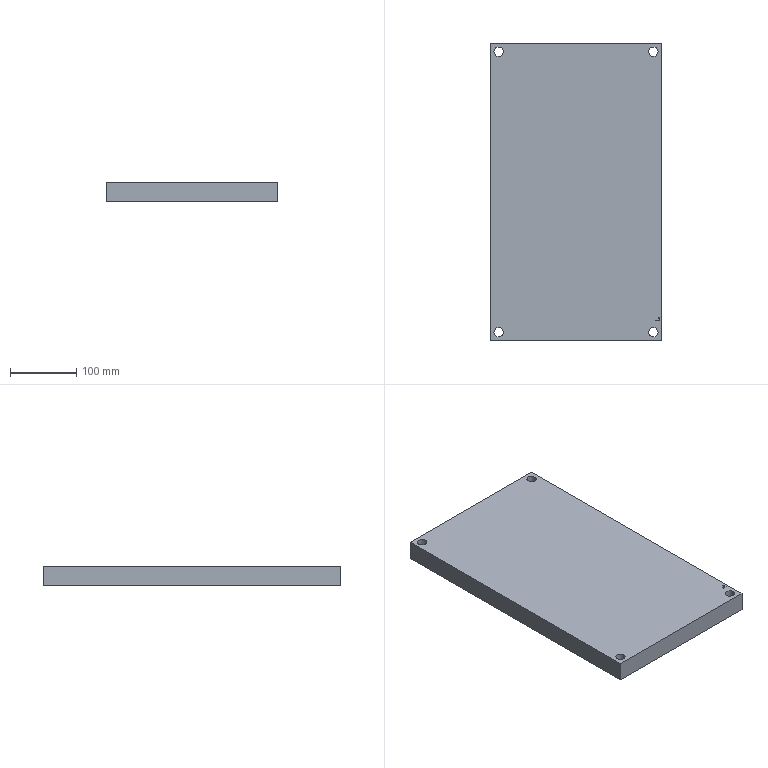Part | NX | features solid 2 | 1 solid | 25 faces | box 260 x 450 x 30 mm | volume 3483194 mm3 | plane 17 | cylinder 8 | commonest cylinder face diameters 14 x4 20 x4
STEP:
#1=CARTESIAN_POINT('',(110.,-212.,-345.5));
#2=VERTEX_POINT('',#1);
#3=CARTESIAN_POINT('',(117.,-212.,-345.5));
#4=DIRECTION('',(0.,0.,-1.));
#5=DIRECTION('',(-1.,0.,0.));
#6=AXIS2_PLACEMENT_3D('',#3,#4,#5);
#7=CIRCLE('',#6,7.);
#8=EDGE_CURVE('',#2,#2,#7,.T.);
#9=ORIENTED_EDGE('',*,*,#8,.T.);
#10=EDGE_LOOP('',(#9));
#11=FACE_BOUND('',#10,.T.);
#12=CARTESIAN_POINT('',(110.,212.,-345.5));
#13=VERTEX_POINT('',#12);
#14=CARTESIAN_POINT('',(117.,212.,-345.5));
#15=DIRECTION('',(0.,0.,-1.));
#16=DIRECTION('',(-1.,0.,0.));
#17=AXIS2_PLACEMENT_3D('',#14,#15,#16);
#18=CIRCLE('',#17,7.);
#19=EDGE_CURVE('',#13,#13,#18,.T.);
#20=ORIENTED_EDGE('',*,*,#19,.T.);
#21=EDGE_LOOP('',(#20));
#22=FACE_BOUND('',#21,.T.);
#23=CARTESIAN_POINT('',(-124.,212.,-345.5));
#24=VERTEX_POINT('',#23);
#25=CARTESIAN_POINT('',(-117.,212.,-345.5));
#26=DIRECTION('',(0.,0.,-1.));
#27=DIRECTION('',(-1.,0.,0.));
#28=AXIS2_PLACEMENT_3D('',#25,#26,#27);
#29=CIRCLE('',#28,7.);
#30=EDGE_CURVE('',#24,#24,#29,.T.);
#31=ORIENTED_EDGE('',*,*,#30,.T.);
#32=EDGE_LOOP('',(#31));
#33=FACE_BOUND('',#32,.T.);
#34=CARTESIAN_POINT('',(-124.,-212.,-345.5));
#35=VERTEX_POINT('',#34);
#36=CARTESIAN_POINT('',(-117.,-212.,-345.5));
#37=DIRECTION('',(0.,0.,-1.));
#38=DIRECTION('',(-1.,0.,0.));
#39=AXIS2_PLACEMENT_3D('',#36,#37,#38);
#40=CIRCLE('',#39,7.);
#41=EDGE_CURVE('',#35,#35,#40,.T.);
#42=ORIENTED_EDGE('',*,*,#41,.T.);
#43=EDGE_LOOP('',(#42));
#44=FACE_BOUND('',#43,.T.);
#45=CARTESIAN_POINT('',(120.4,-195.,-345.5));
#46=VERTEX_POINT('',#45);
#47=CARTESIAN_POINT('',(126.,-195.,-345.5));
#48=VERTEX_POINT('',#47);
#49=CARTESIAN_POINT('',(120.4,-195.,-345.5));
#50=DIRECTION('',(1.,0.,0.));
#51=VECTOR('',#50,1000.);
#52=LINE('',#49,#51);
#53=EDGE_CURVE('',#46,#48,#52,.T.);
#54=ORIENTED_EDGE('',*,*,#53,.F.);
#55=CARTESIAN_POINT('',(120.4,-193.8,-345.5));
#56=VERTEX_POINT('',#55);
#57=CARTESIAN_POINT('',(120.4,-195.,-345.5));
#58=DIRECTION('',(0.,-1.,0.));
#59=VECTOR('',#58,1000.);
#60=LINE('',#57,#59);
#61=EDGE_CURVE('',#56,#46,#60,.T.);
#62=ORIENTED_EDGE('',*,*,#61,.F.);
#63=CARTESIAN_POINT('',(124.8,-193.8,-345.5));
#64=VERTEX_POINT('',#63);
#65=CARTESIAN_POINT('',(120.4,-193.8,-345.5));
#66=DIRECTION('',(-1.,0.,0.));
#67=VECTOR('',#66,1000.);
#68=LINE('',#65,#67);
#69=EDGE_CURVE('',#64,#56,#68,.T.);
#70=ORIENTED_EDGE('',*,*,#69,.F.);
#71=CARTESIAN_POINT('',(124.8,-189.4,-345.5));
#72=VERTEX_POINT('',#71);
#73=CARTESIAN_POINT('',(124.8,-193.8,-345.5));
#74=DIRECTION('',(0.,-1.,0.));
#75=VECTOR('',#74,1000.);
#76=LINE('',#73,#75);
#77=EDGE_CURVE('',#72,#64,#76,.T.);
#78=ORIENTED_EDGE('',*,*,#77,.F.);
#79=CARTESIAN_POINT('',(126.,-189.4,-345.5));
#80=VERTEX_POINT('',#79);
#81=CARTESIAN_POINT('',(124.8,-189.4,-345.5));
#82=DIRECTION('',(-1.,0.,0.));
#83=VECTOR('',#82,1000.);
#84=LINE('',#81,#83);
#85=EDGE_CURVE('',#80,#72,#84,.T.);
#86=ORIENTED_EDGE('',*,*,#85,.F.);
#87=CARTESIAN_POINT('',(126.,-189.4,-345.5));
#88=DIRECTION('',(0.,1.,0.));
#89=VECTOR('',#88,1000.);
#90=LINE('',#87,#89);
#91=EDGE_CURVE('',#48,#80,#90,.T.);
#92=ORIENTED_EDGE('',*,*,#91,.F.);
#93=EDGE_LOOP('',(#54,#62,#70,#78,#86,#92));
#94=FACE_BOUND('',#93,.T.);
#95=CARTESIAN_POINT('',(130.,-225.,-345.5));
#96=VERTEX_POINT('',#95);
#97=CARTESIAN_POINT('',(-130.,-225.,-345.5));
#98=VERTEX_POINT('',#97);
#99=CARTESIAN_POINT('',(0.,-225.,-345.5));
#100=DIRECTION('',(-1.,0.,0.));
#101=VECTOR('',#100,1000.);
#102=LINE('',#99,#101);
#103=EDGE_CURVE('',#96,#98,#102,.T.);
#104=ORIENTED_EDGE('',*,*,#103,.F.);
#105=CARTESIAN_POINT('',(130.,225.,-345.5));
#106=VERTEX_POINT('',#105);
#107=CARTESIAN_POINT('',(130.,0.,-345.5));
#108=DIRECTION('',(0.,-1.,0.));
#109=VECTOR('',#108,1000.);
#110=LINE('',#107,#109);
#111=EDGE_CURVE('',#106,#96,#110,.T.);
#112=ORIENTED_EDGE('',*,*,#111,.F.);
#113=CARTESIAN_POINT('',(-130.,225.,-345.5));
#114=VERTEX_POINT('',#113);
#115=CARTESIAN_POINT('',(0.,225.,-345.5));
#116=DIRECTION('',(1.,0.,0.));
#117=VECTOR('',#116,1000.);
#118=LINE('',#115,#117);
#119=EDGE_CURVE('',#114,#106,#118,.T.);
#120=ORIENTED_EDGE('',*,*,#119,.F.);
#121=CARTESIAN_POINT('',(-130.,0.,-345.5));
#122=DIRECTION('',(0.,1.,0.));
#123=VECTOR('',#122,1000.);
#124=LINE('',#121,#123);
#125=EDGE_CURVE('',#98,#114,#124,.T.);
#126=ORIENTED_EDGE('',*,*,#125,.F.);
#127=EDGE_LOOP('',(#104,#112,#120,#126));
#128=FACE_BOUND('',#127,.T.);
#129=CARTESIAN_POINT('',(0.,0.,-345.5));
#130=DIRECTION('',(0.,0.,1.));
#131=DIRECTION('',(1.,0.,0.));
#132=AXIS2_PLACEMENT_3D('',#129,#130,#131);
#133=PLANE('',#132);
#134=ADVANCED_FACE('',(#11,#22,#33,#44,#94,#128),#133,.T.);
#135=CARTESIAN_POINT('',(130.,-225.,-375.5));
#136=VERTEX_POINT('',#135);
#137=CARTESIAN_POINT('',(130.,-225.,-375.5));
#138=DIRECTION('',(0.,0.,1.));
#139=VECTOR('',#138,1000.);
#140=LINE('',#137,#139);
#141=EDGE_CURVE('',#136,#96,#140,.T.);
#142=ORIENTED_EDGE('',*,*,#141,.T.);
#143=ORIENTED_EDGE('',*,*,#103,.T.);
#144=CARTESIAN_POINT('',(-130.,-225.,-375.5));
#145=VERTEX_POINT('',#144);
#146=CARTESIAN_POINT('',(-130.,-225.,-375.5));
#147=DIRECTION('',(0.,0.,1.));
#148=VECTOR('',#147,1000.);
#149=LINE('',#146,#148);
#150=EDGE_CURVE('',#145,#98,#149,.T.);
#151=ORIENTED_EDGE('',*,*,#150,.F.);
#152=CARTESIAN_POINT('',(0.,-225.,-375.5));
#153=DIRECTION('',(1.,0.,0.));
#154=VECTOR('',#153,1000.);
#155=LINE('',#152,#154);
#156=EDGE_CURVE('',#145,#136,#155,.T.);
#157=ORIENTED_EDGE('',*,*,#156,.T.);
#158=EDGE_LOOP('',(#142,#143,#151,#157));
#159=FACE_BOUND('',#158,.T.);
#160=CARTESIAN_POINT('',(0.,-225.,-375.5));
#161=DIRECTION('',(0.,-1.,0.));
#162=DIRECTION('',(0.,0.,-1.));
#163=AXIS2_PLACEMENT_3D('',#160,#161,#162);
#164=PLANE('',#163);
#165=ADVANCED_FACE('',(#159),#164,.T.);
#166=ORIENTED_EDGE('',*,*,#150,.T.);
#167=ORIENTED_EDGE('',*,*,#125,.T.);
#168=CARTESIAN_POINT('',(-130.,225.,-375.5));
#169=VERTEX_POINT('',#168);
#170=CARTESIAN_POINT('',(-130.,225.,-375.5));
#171=DIRECTION('',(0.,0.,1.));
#172=VECTOR('',#171,1000.);
#173=LINE('',#170,#172);
#174=EDGE_CURVE('',#169,#114,#173,.T.);
#175=ORIENTED_EDGE('',*,*,#174,.F.);
#176=CARTESIAN_POINT('',(-130.,0.,-375.5));
#177=DIRECTION('',(0.,-1.,0.));
#178=VECTOR('',#177,1000.);
#179=LINE('',#176,#178);
#180=EDGE_CURVE('',#169,#145,#179,.T.);
#181=ORIENTED_EDGE('',*,*,#180,.T.);
#182=EDGE_LOOP('',(#166,#167,#175,#181));
#183=FACE_BOUND('',#182,.T.);
#184=CARTESIAN_POINT('',(-130.,0.,-375.5));
#185=DIRECTION('',(-1.,0.,0.));
#186=DIRECTION('',(0.,0.,1.));
#187=AXIS2_PLACEMENT_3D('',#184,#185,#186);
#188=PLANE('',#187);
#189=ADVANCED_FACE('',(#183),#188,.T.);
#190=ORIENTED_EDGE('',*,*,#174,.T.);
#191=ORIENTED_EDGE('',*,*,#119,.T.);
#192=CARTESIAN_POINT('',(130.,225.,-375.5));
#193=VERTEX_POINT('',#192);
#194=CARTESIAN_POINT('',(130.,225.,-375.5));
#195=DIRECTION('',(0.,0.,1.));
#196=VECTOR('',#195,1000.);
#197=LINE('',#194,#196);
#198=EDGE_CURVE('',#193,#106,#197,.T.);
#199=ORIENTED_EDGE('',*,*,#198,.F.);
#200=CARTESIAN_POINT('',(0.,225.,-375.5));
#201=DIRECTION('',(-1.,0.,0.));
#202=VECTOR('',#201,1000.);
#203=LINE('',#200,#202);
#204=EDGE_CURVE('',#193,#169,#203,.T.);
#205=ORIENTED_EDGE('',*,*,#204,.T.);
#206=EDGE_LOOP('',(#190,#191,#199,#205));
#207=FACE_BOUND('',#206,.T.);
#208=CARTESIAN_POINT('',(0.,225.,-375.5));
#209=DIRECTION('',(0.,1.,0.));
#210=DIRECTION('',(0.,0.,1.));
#211=AXIS2_PLACEMENT_3D('',#208,#209,#210);
#212=PLANE('',#211);
#213=ADVANCED_FACE('',(#207),#212,.T.);
#214=CARTESIAN_POINT('',(107.,-212.,-375.5));
#215=VERTEX_POINT('',#214);
#216=CARTESIAN_POINT('',(117.,-212.,-375.5));
#217=DIRECTION('',(0.,0.,1.));
#218=DIRECTION('',(-1.,0.,0.));
#219=AXIS2_PLACEMENT_3D('',#216,#217,#218);
#220=CIRCLE('',#219,10.);
#221=EDGE_CURVE('',#215,#215,#220,.T.);
#222=ORIENTED_EDGE('',*,*,#221,.T.);
#223=EDGE_LOOP('',(#222));
#224=FACE_BOUND('',#223,.T.);
#225=CARTESIAN_POINT('',(107.,212.,-375.5));
#226=VERTEX_POINT('',#225);
#227=CARTESIAN_POINT('',(117.,212.,-375.5));
#228=DIRECTION('',(0.,0.,1.));
#229=DIRECTION('',(-1.,0.,0.));
#230=AXIS2_PLACEMENT_3D('',#227,#228,#229);
#231=CIRCLE('',#230,10.);
#232=EDGE_CURVE('',#226,#226,#231,.T.);
#233=ORIENTED_EDGE('',*,*,#232,.T.);
#234=EDGE_LOOP('',(#233));
#235=FACE_BOUND('',#234,.T.);
#236=CARTESIAN_POINT('',(-127.,212.,-375.5));
#237=VERTEX_POINT('',#236);
#238=CARTESIAN_POINT('',(-117.,212.,-375.5));
#239=DIRECTION('',(0.,0.,1.));
#240=DIRECTION('',(-1.,0.,0.));
#241=AXIS2_PLACEMENT_3D('',#238,#239,#240);
#242=CIRCLE('',#241,10.);
#243=EDGE_CURVE('',#237,#237,#242,.T.);
#244=ORIENTED_EDGE('',*,*,#243,.T.);
#245=EDGE_LOOP('',(#244));
#246=FACE_BOUND('',#245,.T.);
#247=CARTESIAN_POINT('',(-127.,-212.,-375.5));
#248=VERTEX_POINT('',#247);
#249=CARTESIAN_POINT('',(-117.,-212.,-375.5));
#250=DIRECTION('',(0.,0.,1.));
#251=DIRECTION('',(-1.,0.,0.));
#252=AXIS2_PLACEMENT_3D('',#249,#250,#251);
#253=CIRCLE('',#252,10.);
#254=EDGE_CURVE('',#248,#248,#253,.T.);
#255=ORIENTED_EDGE('',*,*,#254,.T.);
#256=EDGE_LOOP('',(#255));
#257=FACE_BOUND('',#256,.T.);
#258=CARTESIAN_POINT('',(130.,0.,-375.5));
#259=DIRECTION('',(0.,1.,0.));
#260=VECTOR('',#259,1000.);
#261=LINE('',#258,#260);
#262=EDGE_CURVE('',#136,#193,#261,.T.);
#263=ORIENTED_EDGE('',*,*,#262,.F.);
#264=ORIENTED_EDGE('',*,*,#156,.F.);
#265=ORIENTED_EDGE('',*,*,#180,.F.);
#266=ORIENTED_EDGE('',*,*,#204,.F.);
#267=EDGE_LOOP('',(#263,#264,#265,#266));
#268=FACE_BOUND('',#267,.T.);
#269=CARTESIAN_POINT('',(0.,0.,-375.5));
#270=DIRECTION('',(0.,0.,-1.));
#271=DIRECTION('',(-1.,0.,0.));
#272=AXIS2_PLACEMENT_3D('',#269,#270,#271);
#273=PLANE('',#272);
#274=ADVANCED_FACE('',(#224,#235,#246,#257,#268),#273,.T.);
#275=ORIENTED_EDGE('',*,*,#262,.T.);
#276=ORIENTED_EDGE('',*,*,#198,.T.);
#277=ORIENTED_EDGE('',*,*,#111,.T.);
#278=ORIENTED_EDGE('',*,*,#141,.F.);
#279=EDGE_LOOP('',(#275,#276,#277,#278));
#280=FACE_BOUND('',#279,.T.);
#281=CARTESIAN_POINT('',(130.,0.,-375.5));
#282=DIRECTION('',(1.,0.,0.));
#283=DIRECTION('',(0.,0.,-1.));
#284=AXIS2_PLACEMENT_3D('',#281,#282,#283);
#285=PLANE('',#284);
#286=ADVANCED_FACE('',(#280),#285,.T.);
#287=ORIENTED_EDGE('',*,*,#53,.T.);
#288=CARTESIAN_POINT('',(126.,-195.,-345.65));
#289=VERTEX_POINT('',#288);
#290=CARTESIAN_POINT('',(126.,-195.,-345.65));
#291=DIRECTION('',(0.,0.,1.));
#292=VECTOR('',#291,1000.);
#293=LINE('',#290,#292);
#294=EDGE_CURVE('',#289,#48,#293,.T.);
#295=ORIENTED_EDGE('',*,*,#294,.F.);
#296=CARTESIAN_POINT('',(120.4,-195.,-345.65));
#297=VERTEX_POINT('',#296);
#298=CARTESIAN_POINT('',(120.4,-195.,-345.65));
#299=DIRECTION('',(1.,0.,0.));
#300=VECTOR('',#299,1000.);
#301=LINE('',#298,#300);
#302=EDGE_CURVE('',#297,#289,#301,.T.);
#303=ORIENTED_EDGE('',*,*,#302,.F.);
#304=CARTESIAN_POINT('',(120.4,-195.,-345.65));
#305=DIRECTION('',(0.,0.,1.));
#306=VECTOR('',#305,1000.);
#307=LINE('',#304,#306);
#308=EDGE_CURVE('',#297,#46,#307,.T.);
#309=ORIENTED_EDGE('',*,*,#308,.T.);
#310=EDGE_LOOP('',(#287,#295,#303,#309));
#311=FACE_BOUND('',#310,.T.);
#312=CARTESIAN_POINT('',(120.4,-195.,-345.65));
#313=DIRECTION('',(0.,-1.,0.));
#314=DIRECTION('',(0.,0.,-1.));
#315=AXIS2_PLACEMENT_3D('',#312,#313,#314);
#316=PLANE('',#315);
#317=ADVANCED_FACE('',(#311),#316,.F.);
#318=ORIENTED_EDGE('',*,*,#91,.T.);
#319=CARTESIAN_POINT('',(126.,-189.4,-345.65));
#320=VERTEX_POINT('',#319);
#321=CARTESIAN_POINT('',(126.,-189.4,-345.65));
#322=DIRECTION('',(0.,0.,1.));
#323=VECTOR('',#322,1000.);
#324=LINE('',#321,#323);
#325=EDGE_CURVE('',#320,#80,#324,.T.);
#326=ORIENTED_EDGE('',*,*,#325,.F.);
#327=CARTESIAN_POINT('',(126.,-189.4,-345.65));
#328=DIRECTION('',(0.,1.,0.));
#329=VECTOR('',#328,1000.);
#330=LINE('',#327,#329);
#331=EDGE_CURVE('',#289,#320,#330,.T.);
#332=ORIENTED_EDGE('',*,*,#331,.F.);
#333=ORIENTED_EDGE('',*,*,#294,.T.);
#334=EDGE_LOOP('',(#318,#326,#332,#333));
#335=FACE_BOUND('',#334,.T.);
#336=CARTESIAN_POINT('',(126.,-189.4,-345.65));
#337=DIRECTION('',(1.,0.,0.));
#338=DIRECTION('',(0.,0.,-1.));
#339=AXIS2_PLACEMENT_3D('',#336,#337,#338);
#340=PLANE('',#339);
#341=ADVANCED_FACE('',(#335),#340,.F.);
#342=ORIENTED_EDGE('',*,*,#85,.T.);
#343=CARTESIAN_POINT('',(124.8,-189.4,-345.65));
#344=VERTEX_POINT('',#343);
#345=CARTESIAN_POINT('',(124.8,-189.4,-345.65));
#346=DIRECTION('',(0.,0.,1.));
#347=VECTOR('',#346,1000.);
#348=LINE('',#345,#347);
#349=EDGE_CURVE('',#344,#72,#348,.T.);
#350=ORIENTED_EDGE('',*,*,#349,.F.);
#351=CARTESIAN_POINT('',(124.8,-189.4,-345.65));
#352=DIRECTION('',(-1.,0.,0.));
#353=VECTOR('',#352,1000.);
#354=LINE('',#351,#353);
#355=EDGE_CURVE('',#320,#344,#354,.T.);
#356=ORIENTED_EDGE('',*,*,#355,.F.);
#357=ORIENTED_EDGE('',*,*,#325,.T.);
#358=EDGE_LOOP('',(#342,#350,#356,#357));
#359=FACE_BOUND('',#358,.T.);
#360=CARTESIAN_POINT('',(124.8,-189.4,-345.65));
#361=DIRECTION('',(0.,1.,0.));
#362=DIRECTION('',(0.,0.,1.));
#363=AXIS2_PLACEMENT_3D('',#360,#361,#362);
#364=PLANE('',#363);
#365=ADVANCED_FACE('',(#359),#364,.F.);
#366=ORIENTED_EDGE('',*,*,#77,.T.);
#367=CARTESIAN_POINT('',(124.8,-193.8,-345.65));
#368=VERTEX_POINT('',#367);
#369=CARTESIAN_POINT('',(124.8,-193.8,-345.65));
#370=DIRECTION('',(0.,0.,1.));
#371=VECTOR('',#370,1000.);
#372=LINE('',#369,#371);
#373=EDGE_CURVE('',#368,#64,#372,.T.);
#374=ORIENTED_EDGE('',*,*,#373,.F.);
#375=CARTESIAN_POINT('',(124.8,-193.8,-345.65));
#376=DIRECTION('',(0.,-1.,0.));
#377=VECTOR('',#376,1000.);
#378=LINE('',#375,#377);
#379=EDGE_CURVE('',#344,#368,#378,.T.);
#380=ORIENTED_EDGE('',*,*,#379,.F.);
#381=ORIENTED_EDGE('',*,*,#349,.T.);
#382=EDGE_LOOP('',(#366,#374,#380,#381));
#383=FACE_BOUND('',#382,.T.);
#384=CARTESIAN_POINT('',(124.8,-193.8,-345.65));
#385=DIRECTION('',(-1.,0.,0.));
#386=DIRECTION('',(0.,0.,1.));
#387=AXIS2_PLACEMENT_3D('',#384,#385,#386);
#388=PLANE('',#387);
#389=ADVANCED_FACE('',(#383),#388,.F.);
#390=ORIENTED_EDGE('',*,*,#69,.T.);
#391=CARTESIAN_POINT('',(120.4,-193.8,-345.65));
#392=VERTEX_POINT('',#391);
#393=CARTESIAN_POINT('',(120.4,-193.8,-345.65));
#394=DIRECTION('',(0.,0.,1.));
#395=VECTOR('',#394,1000.);
#396=LINE('',#393,#395);
#397=EDGE_CURVE('',#392,#56,#396,.T.);
#398=ORIENTED_EDGE('',*,*,#397,.F.);
#399=CARTESIAN_POINT('',(120.4,-193.8,-345.65));
#400=DIRECTION('',(-1.,0.,0.));
#401=VECTOR('',#400,1000.);
#402=LINE('',#399,#401);
#403=EDGE_CURVE('',#368,#392,#402,.T.);
#404=ORIENTED_EDGE('',*,*,#403,.F.);
#405=ORIENTED_EDGE('',*,*,#373,.T.);
#406=EDGE_LOOP('',(#390,#398,#404,#405));
#407=FACE_BOUND('',#406,.T.);
#408=CARTESIAN_POINT('',(120.4,-193.8,-345.65));
#409=DIRECTION('',(0.,1.,0.));
#410=DIRECTION('',(0.,0.,1.));
#411=AXIS2_PLACEMENT_3D('',#408,#409,#410);
#412=PLANE('',#411);
#413=ADVANCED_FACE('',(#407),#412,.F.);
#414=ORIENTED_EDGE('',*,*,#61,.T.);
#415=ORIENTED_EDGE('',*,*,#308,.F.);
#416=CARTESIAN_POINT('',(120.4,-195.,-345.65));
#417=DIRECTION('',(0.,-1.,0.));
#418=VECTOR('',#417,1000.);
#419=LINE('',#416,#418);
#420=EDGE_CURVE('',#392,#297,#419,.T.);
#421=ORIENTED_EDGE('',*,*,#420,.F.);
#422=ORIENTED_EDGE('',*,*,#397,.T.);
#423=EDGE_LOOP('',(#414,#415,#421,#422));
#424=FACE_BOUND('',#423,.T.);
#425=CARTESIAN_POINT('',(120.4,-195.,-345.65));
#426=DIRECTION('',(-1.,0.,0.));
#427=DIRECTION('',(0.,0.,1.));
#428=AXIS2_PLACEMENT_3D('',#425,#426,#427);
#429=PLANE('',#428);
#430=ADVANCED_FACE('',(#424),#429,.F.);
#431=ORIENTED_EDGE('',*,*,#302,.T.);
#432=ORIENTED_EDGE('',*,*,#331,.T.);
#433=ORIENTED_EDGE('',*,*,#355,.T.);
#434=ORIENTED_EDGE('',*,*,#379,.T.);
#435=ORIENTED_EDGE('',*,*,#403,.T.);
#436=ORIENTED_EDGE('',*,*,#420,.T.);
#437=EDGE_LOOP('',(#431,#432,#433,#434,#435,#436));
#438=FACE_BOUND('',#437,.T.);
#439=CARTESIAN_POINT('',(126.,-195.,-345.65));
#440=DIRECTION('',(0.,0.,1.));
#441=DIRECTION('',(1.,0.,0.));
#442=AXIS2_PLACEMENT_3D('',#439,#440,#441);
#443=PLANE('',#442);
#444=ADVANCED_FACE('',(#438),#443,.T.);
#445=CARTESIAN_POINT('',(-110.,-212.,-362.5));
#446=VERTEX_POINT('',#445);
#447=CARTESIAN_POINT('',(-117.,-212.,-362.5));
#448=DIRECTION('',(0.,0.,1.));
#449=DIRECTION('',(1.,0.,0.));
#450=AXIS2_PLACEMENT_3D('',#447,#448,#449);
#451=CIRCLE('',#450,7.);
#452=EDGE_CURVE('',#446,#446,#451,.F.);
#453=ORIENTED_EDGE('',*,*,#452,.T.);
#454=EDGE_LOOP('',(#453));
#455=FACE_BOUND('',#454,.T.);
#456=ORIENTED_EDGE('',*,*,#41,.F.);
#457=EDGE_LOOP('',(#456));
#458=FACE_BOUND('',#457,.T.);
#459=CARTESIAN_POINT('',(-117.,-212.,-345.5));
#460=DIRECTION('',(0.,0.,-1.));
#461=DIRECTION('',(-1.,0.,0.));
#462=AXIS2_PLACEMENT_3D('',#459,#460,#461);
#463=CYLINDRICAL_SURFACE('',#462,7.);
#464=ADVANCED_FACE('',(#455,#458),#463,.F.);
#465=ORIENTED_EDGE('',*,*,#452,.F.);
#466=EDGE_LOOP('',(#465));
#467=FACE_BOUND('',#466,.T.);
#468=CARTESIAN_POINT('',(-127.,-212.,-362.5));
#469=VERTEX_POINT('',#468);
#470=CARTESIAN_POINT('',(-117.,-212.,-362.5));
#471=DIRECTION('',(0.,0.,-1.));
#472=DIRECTION('',(-1.,0.,0.));
#473=AXIS2_PLACEMENT_3D('',#470,#471,#472);
#474=CIRCLE('',#473,10.);
#475=EDGE_CURVE('',#469,#469,#474,.T.);
#476=ORIENTED_EDGE('',*,*,#475,.T.);
#477=EDGE_LOOP('',(#476));
#478=FACE_BOUND('',#477,.T.);
#479=CARTESIAN_POINT('',(-117.,-212.,-362.5));
#480=DIRECTION('',(0.,0.,1.));
#481=DIRECTION('',(1.,0.,0.));
#482=AXIS2_PLACEMENT_3D('',#479,#480,#481);
#483=PLANE('',#482);
#484=ADVANCED_FACE('',(#467,#478),#483,.F.);
#485=ORIENTED_EDGE('',*,*,#254,.F.);
#486=EDGE_LOOP('',(#485));
#487=FACE_BOUND('',#486,.T.);
#488=ORIENTED_EDGE('',*,*,#475,.F.);
#489=EDGE_LOOP('',(#488));
#490=FACE_BOUND('',#489,.T.);
#491=CARTESIAN_POINT('',(-117.,-212.,-362.5));
#492=DIRECTION('',(0.,0.,-1.));
#493=DIRECTION('',(-1.,0.,0.));
#494=AXIS2_PLACEMENT_3D('',#491,#492,#493);
#495=CYLINDRICAL_SURFACE('',#494,10.);
#496=ADVANCED_FACE('',(#487,#490),#495,.F.);
#497=CARTESIAN_POINT('',(-110.,212.,-362.5));
#498=VERTEX_POINT('',#497);
#499=CARTESIAN_POINT('',(-117.,212.,-362.5));
#500=DIRECTION('',(0.,0.,1.));
#501=DIRECTION('',(1.,0.,0.));
#502=AXIS2_PLACEMENT_3D('',#499,#500,#501);
#503=CIRCLE('',#502,7.);
#504=EDGE_CURVE('',#498,#498,#503,.F.);
#505=ORIENTED_EDGE('',*,*,#504,.T.);
#506=EDGE_LOOP('',(#505));
#507=FACE_BOUND('',#506,.T.);
#508=ORIENTED_EDGE('',*,*,#30,.F.);
#509=EDGE_LOOP('',(#508));
#510=FACE_BOUND('',#509,.T.);
#511=CARTESIAN_POINT('',(-117.,212.,-345.5));
#512=DIRECTION('',(0.,0.,-1.));
#513=DIRECTION('',(-1.,0.,0.));
#514=AXIS2_PLACEMENT_3D('',#511,#512,#513);
#515=CYLINDRICAL_SURFACE('',#514,7.);
#516=ADVANCED_FACE('',(#507,#510),#515,.F.);
#517=ORIENTED_EDGE('',*,*,#504,.F.);
#518=EDGE_LOOP('',(#517));
#519=FACE_BOUND('',#518,.T.);
#520=CARTESIAN_POINT('',(-127.,212.,-362.5));
#521=VERTEX_POINT('',#520);
#522=CARTESIAN_POINT('',(-117.,212.,-362.5));
#523=DIRECTION('',(0.,0.,-1.));
#524=DIRECTION('',(-1.,0.,0.));
#525=AXIS2_PLACEMENT_3D('',#522,#523,#524);
#526=CIRCLE('',#525,10.);
#527=EDGE_CURVE('',#521,#521,#526,.T.);
#528=ORIENTED_EDGE('',*,*,#527,.T.);
#529=EDGE_LOOP('',(#528));
#530=FACE_BOUND('',#529,.T.);
#531=CARTESIAN_POINT('',(-117.,212.,-362.5));
#532=DIRECTION('',(0.,0.,1.));
#533=DIRECTION('',(1.,0.,0.));
#534=AXIS2_PLACEMENT_3D('',#531,#532,#533);
#535=PLANE('',#534);
#536=ADVANCED_FACE('',(#519,#530),#535,.F.);
#537=ORIENTED_EDGE('',*,*,#243,.F.);
#538=EDGE_LOOP('',(#537));
#539=FACE_BOUND('',#538,.T.);
#540=ORIENTED_EDGE('',*,*,#527,.F.);
#541=EDGE_LOOP('',(#540));
#542=FACE_BOUND('',#541,.T.);
#543=CARTESIAN_POINT('',(-117.,212.,-362.5));
#544=DIRECTION('',(0.,0.,-1.));
#545=DIRECTION('',(-1.,0.,0.));
#546=AXIS2_PLACEMENT_3D('',#543,#544,#545);
#547=CYLINDRICAL_SURFACE('',#546,10.);
#548=ADVANCED_FACE('',(#539,#542),#547,.F.);
#549=CARTESIAN_POINT('',(124.,212.,-362.5));
#550=VERTEX_POINT('',#549);
#551=CARTESIAN_POINT('',(117.,212.,-362.5));
#552=DIRECTION('',(0.,0.,1.));
#553=DIRECTION('',(1.,0.,0.));
#554=AXIS2_PLACEMENT_3D('',#551,#552,#553);
#555=CIRCLE('',#554,7.);
#556=EDGE_CURVE('',#550,#550,#555,.F.);
#557=ORIENTED_EDGE('',*,*,#556,.T.);
#558=EDGE_LOOP('',(#557));
#559=FACE_BOUND('',#558,.T.);
#560=ORIENTED_EDGE('',*,*,#19,.F.);
#561=EDGE_LOOP('',(#560));
#562=FACE_BOUND('',#561,.T.);
#563=CARTESIAN_POINT('',(117.,212.,-345.5));
#564=DIRECTION('',(0.,0.,-1.));
#565=DIRECTION('',(-1.,0.,0.));
#566=AXIS2_PLACEMENT_3D('',#563,#564,#565);
#567=CYLINDRICAL_SURFACE('',#566,7.);
#568=ADVANCED_FACE('',(#559,#562),#567,.F.);
#569=ORIENTED_EDGE('',*,*,#556,.F.);
#570=EDGE_LOOP('',(#569));
#571=FACE_BOUND('',#570,.T.);
#572=CARTESIAN_POINT('',(107.,212.,-362.5));
#573=VERTEX_POINT('',#572);
#574=CARTESIAN_POINT('',(117.,212.,-362.5));
#575=DIRECTION('',(0.,0.,-1.));
#576=DIRECTION('',(-1.,0.,0.));
#577=AXIS2_PLACEMENT_3D('',#574,#575,#576);
#578=CIRCLE('',#577,10.);
#579=EDGE_CURVE('',#573,#573,#578,.T.);
#580=ORIENTED_EDGE('',*,*,#579,.T.);
#581=EDGE_LOOP('',(#580));
#582=FACE_BOUND('',#581,.T.);
#583=CARTESIAN_POINT('',(117.,212.,-362.5));
#584=DIRECTION('',(0.,0.,1.));
#585=DIRECTION('',(1.,0.,0.));
#586=AXIS2_PLACEMENT_3D('',#583,#584,#585);
#587=PLANE('',#586);
#588=ADVANCED_FACE('',(#571,#582),#587,.F.);
#589=ORIENTED_EDGE('',*,*,#232,.F.);
#590=EDGE_LOOP('',(#589));
#591=FACE_BOUND('',#590,.T.);
#592=ORIENTED_EDGE('',*,*,#579,.F.);
#593=EDGE_LOOP('',(#592));
#594=FACE_BOUND('',#593,.T.);
#595=CARTESIAN_POINT('',(117.,212.,-362.5));
#596=DIRECTION('',(0.,0.,-1.));
#597=DIRECTION('',(-1.,0.,0.));
#598=AXIS2_PLACEMENT_3D('',#595,#596,#597);
#599=CYLINDRICAL_SURFACE('',#598,10.);
#600=ADVANCED_FACE('',(#591,#594),#599,.F.);
#601=CARTESIAN_POINT('',(124.,-212.,-362.5));
#602=VERTEX_POINT('',#601);
#603=CARTESIAN_POINT('',(117.,-212.,-362.5));
#604=DIRECTION('',(0.,0.,1.));
#605=DIRECTION('',(1.,0.,0.));
#606=AXIS2_PLACEMENT_3D('',#603,#604,#605);
#607=CIRCLE('',#606,7.);
#608=EDGE_CURVE('',#602,#602,#607,.F.);
#609=ORIENTED_EDGE('',*,*,#608,.T.);
#610=EDGE_LOOP('',(#609));
#611=FACE_BOUND('',#610,.T.);
#612=ORIENTED_EDGE('',*,*,#8,.F.);
#613=EDGE_LOOP('',(#612));
#614=FACE_BOUND('',#613,.T.);
#615=CARTESIAN_POINT('',(117.,-212.,-345.5));
#616=DIRECTION('',(0.,0.,-1.));
#617=DIRECTION('',(-1.,0.,0.));
#618=AXIS2_PLACEMENT_3D('',#615,#616,#617);
#619=CYLINDRICAL_SURFACE('',#618,7.);
#620=ADVANCED_FACE('',(#611,#614),#619,.F.);
#621=ORIENTED_EDGE('',*,*,#608,.F.);
#622=EDGE_LOOP('',(#621));
#623=FACE_BOUND('',#622,.T.);
#624=CARTESIAN_POINT('',(107.,-212.,-362.5));
#625=VERTEX_POINT('',#624);
#626=CARTESIAN_POINT('',(117.,-212.,-362.5));
#627=DIRECTION('',(0.,0.,-1.));
#628=DIRECTION('',(-1.,0.,0.));
#629=AXIS2_PLACEMENT_3D('',#626,#627,#628);
#630=CIRCLE('',#629,10.);
#631=EDGE_CURVE('',#625,#625,#630,.T.);
#632=ORIENTED_EDGE('',*,*,#631,.T.);
#633=EDGE_LOOP('',(#632));
#634=FACE_BOUND('',#633,.T.);
#635=CARTESIAN_POINT('',(117.,-212.,-362.5));
#636=DIRECTION('',(0.,0.,1.));
#637=DIRECTION('',(1.,0.,0.));
#638=AXIS2_PLACEMENT_3D('',#635,#636,#637);
#639=PLANE('',#638);
#640=ADVANCED_FACE('',(#623,#634),#639,.F.);
#641=ORIENTED_EDGE('',*,*,#221,.F.);
#642=EDGE_LOOP('',(#641));
#643=FACE_BOUND('',#642,.T.);
#644=ORIENTED_EDGE('',*,*,#631,.F.);
#645=EDGE_LOOP('',(#644));
#646=FACE_BOUND('',#645,.T.);
#647=CARTESIAN_POINT('',(117.,-212.,-362.5));
#648=DIRECTION('',(0.,0.,-1.));
#649=DIRECTION('',(-1.,0.,0.));
#650=AXIS2_PLACEMENT_3D('',#647,#648,#649);
#651=CYLINDRICAL_SURFACE('',#650,10.);
#652=ADVANCED_FACE('',(#643,#646),#651,.F.);
#653=CLOSED_SHELL('',(#134,#165,#189,#213,#274,#286,#317,#341,#365,#389,#413,#430,#444,#464,#484,#496,#516,#536,#548,#568,#588,#600,#620,#640,#652));
#654=MANIFOLD_SOLID_BREP('',#653);
#655=(LENGTH_UNIT()NAMED_UNIT(*)SI_UNIT(.MILLI.,.METRE.));
#656=UNCERTAINTY_MEASURE_WITH_UNIT(LENGTH_MEASURE(0.00001),#655,'','');
#657=(NAMED_UNIT(*)PLANE_ANGLE_UNIT()SI_UNIT($,.RADIAN.));
#658=(NAMED_UNIT(*)SI_UNIT($,.STERADIAN.)SOLID_ANGLE_UNIT());
#659=(GEOMETRIC_REPRESENTATION_CONTEXT(3)GLOBAL_UNCERTAINTY_ASSIGNED_CONTEXT((#656))GLOBAL_UNIT_ASSIGNED_CONTEXT((#655,#657,#658))REPRESENTATION_CONTEXT('',''));
#660=ADVANCED_BREP_SHAPE_REPRESENTATION('',(#654),#659);